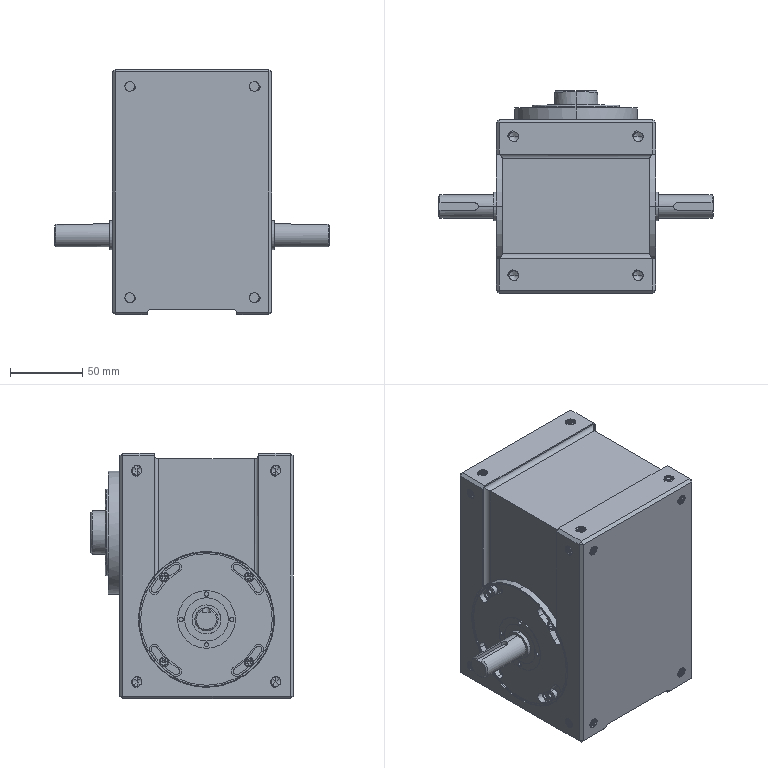Part | STEP file | 60DF cam indexer | 11 solids | 1618 faces | box 190 x 140 x 170 mm | volume 2161358 mm3 | cylinder 730 | plane 572 | spline 281 | cone 35 | commonest cylinder face diameters 6.8 x403 5 x143 4.5 x24 7 x24 3 x16 4 x16